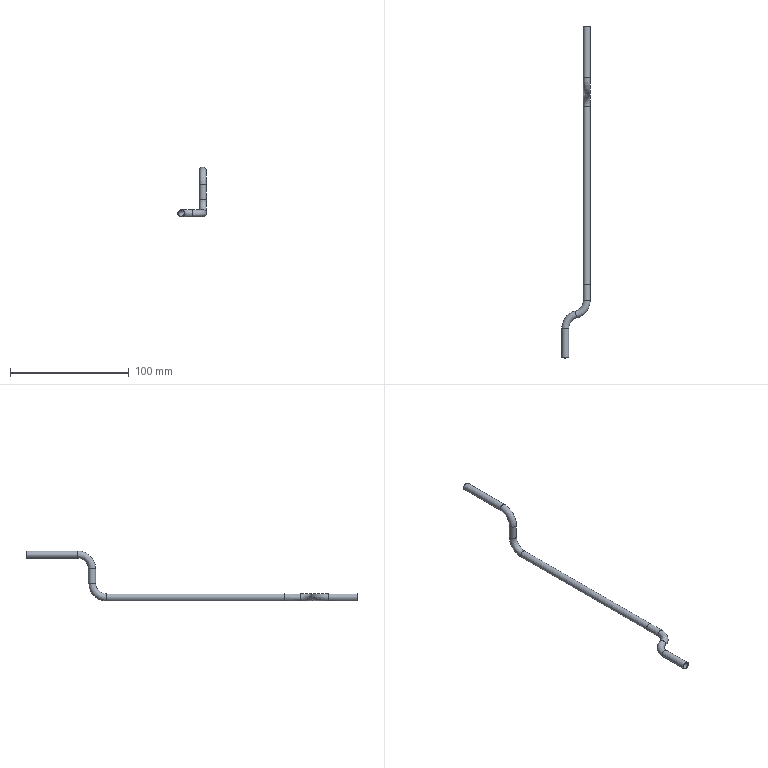Part | STEP file | 1-72 | 1 solid | 20 faces | box 24 x 279.352 x 42 mm | volume 2708 mm3 | cylinder 10 | torus 8 | plane 2 | commonest cylinder face diameters 5 x5 6 x5